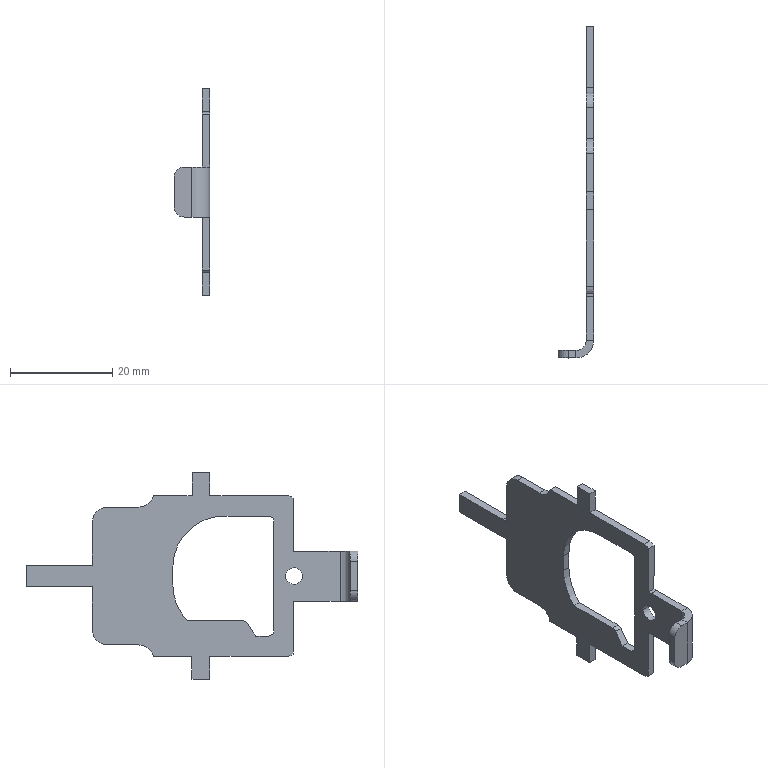Part | SolidWorks | features BaseBody 1 | 1 solid | 57 faces | box 7.018 x 65.003 x 40.503 mm | volume 1553 mm3 | plane 40 | cylinder 17 | commonest cylinder face diameters 4 x5 6 x4 2 x3 3.3 x2 20 x2 7 x1